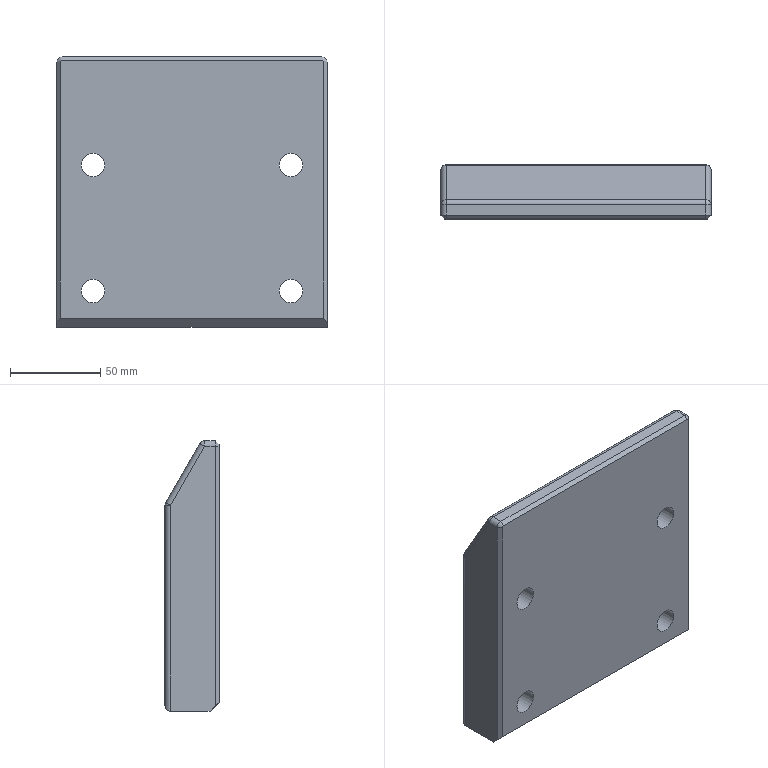Part | NX | features solid 2 | 1 solid | 42 faces | box 150 x 30 x 150 mm | volume 590878 mm3 | cylinder 17 | plane 15 | torus 4 | sphere 4 | cone 2 | commonest cylinder face diameters 6 x9 13 x4 20 x4
STEP:
#1=CARTESIAN_POINT('',(-235.5,-600.,-133.));
#2=VERTEX_POINT('',#1);
#3=CARTESIAN_POINT('',(-235.5,-600.,-275.));
#4=VERTEX_POINT('',#3);
#5=CARTESIAN_POINT('',(-235.5,-600.,-170.));
#6=DIRECTION('',(0.,0.,-1.));
#7=VECTOR('',#6,1000.);
#8=LINE('',#5,#7);
#9=EDGE_CURVE('',#2,#4,#8,.T.);
#10=ORIENTED_EDGE('',*,*,#9,.T.);
#11=CARTESIAN_POINT('',(-233.5,-598.,-277.));
#12=VERTEX_POINT('',#11);
#13=CARTESIAN_POINT('',(-277.167,-641.667,-233.333));
#14=DIRECTION('',(0.5774,0.5774,-0.5774));
#15=VECTOR('',#14,1000.);
#16=LINE('',#13,#15);
#17=EDGE_CURVE('',#12,#4,#16,.F.);
#18=ORIENTED_EDGE('',*,*,#17,.F.);
#19=CARTESIAN_POINT('',(-233.5,-598.,-133.));
#20=VERTEX_POINT('',#19);
#21=CARTESIAN_POINT('',(-233.5,-598.,-43.));
#22=DIRECTION('',(0.,0.,1.));
#23=VECTOR('',#22,1000.);
#24=LINE('',#21,#23);
#25=EDGE_CURVE('',#12,#20,#24,.T.);
#26=ORIENTED_EDGE('',*,*,#25,.T.);
#27=CARTESIAN_POINT('',(-233.5,-598.,-133.));
#28=DIRECTION('',(-0.7071,-0.7071,0.));
#29=VECTOR('',#28,1000.);
#30=LINE('',#27,#29);
#31=EDGE_CURVE('',#20,#2,#30,.T.);
#32=ORIENTED_EDGE('',*,*,#31,.T.);
#33=EDGE_LOOP('',(#10,#18,#26,#32));
#34=FACE_BOUND('',#33,.T.);
#35=CARTESIAN_POINT('',(-235.5,-600.,-40.));
#36=DIRECTION('',(0.7071,-0.7071,0.));
#37=DIRECTION('',(-0.7071,-0.7071,0.));
#38=AXIS2_PLACEMENT_3D('',#35,#36,#37);
#39=PLANE('',#38);
#40=ADVANCED_FACE('',(#34),#39,.T.);
#41=CARTESIAN_POINT('',(-233.5,-573.,-165.804));
#42=VERTEX_POINT('',#41);
#43=CARTESIAN_POINT('',(-233.5,-573.,-280.));
#44=VERTEX_POINT('',#43);
#45=CARTESIAN_POINT('',(-233.5,-573.,-170.));
#46=DIRECTION('',(0.,0.,1.));
#47=VECTOR('',#46,1000.);
#48=LINE('',#45,#47);
#49=EDGE_CURVE('',#42,#44,#48,.F.);
#50=ORIENTED_EDGE('',*,*,#49,.T.);
#51=CARTESIAN_POINT('',(-236.5,-570.,-277.));
#52=VERTEX_POINT('',#51);
#53=CARTESIAN_POINT('',(-236.5,-573.,-277.));
#54=DIRECTION('',(0.7071,0.,0.7071));
#55=DIRECTION('',(-0.7071,0.,0.7071));
#56=AXIS2_PLACEMENT_3D('',#53,#54,#55);
#57=ELLIPSE('',#56,4.243,3.);
#58=EDGE_CURVE('',#44,#52,#57,.T.);
#59=ORIENTED_EDGE('',*,*,#58,.T.);
#60=CARTESIAN_POINT('',(-236.5,-570.,-165.804));
#61=VERTEX_POINT('',#60);
#62=CARTESIAN_POINT('',(-236.5,-570.,-75.));
#63=DIRECTION('',(0.,0.,1.));
#64=VECTOR('',#63,1000.);
#65=LINE('',#62,#64);
#66=EDGE_CURVE('',#52,#61,#65,.T.);
#67=ORIENTED_EDGE('',*,*,#66,.T.);
#68=CARTESIAN_POINT('',(-236.5,-573.,-165.804));
#69=DIRECTION('',(0.,0.,-1.));
#70=DIRECTION('',(-1.,0.,0.));
#71=AXIS2_PLACEMENT_3D('',#68,#69,#70);
#72=CIRCLE('',#71,3.);
#73=EDGE_CURVE('',#42,#61,#72,.F.);
#74=ORIENTED_EDGE('',*,*,#73,.F.);
#75=EDGE_LOOP('',(#50,#59,#67,#74));
#76=FACE_BOUND('',#75,.T.);
#77=CARTESIAN_POINT('',(-236.5,-573.,-170.));
#78=DIRECTION('',(0.,0.,-1.));
#79=DIRECTION('',(1.,0.,0.));
#80=AXIS2_PLACEMENT_3D('',#77,#78,#79);
#81=CYLINDRICAL_SURFACE('',#80,3.);
#82=ADVANCED_FACE('',(#76),#81,.T.);
#83=ORIENTED_EDGE('',*,*,#25,.F.);
#84=CARTESIAN_POINT('',(-233.5,-595.,-280.));
#85=VERTEX_POINT('',#84);
#86=CARTESIAN_POINT('',(-233.5,-600.,-275.));
#87=DIRECTION('',(0.,0.7071,-0.7071));
#88=VECTOR('',#87,1000.);
#89=LINE('',#86,#88);
#90=EDGE_CURVE('',#85,#12,#89,.F.);
#91=ORIENTED_EDGE('',*,*,#90,.F.);
#92=CARTESIAN_POINT('',(-233.5,-600.,-280.));
#93=DIRECTION('',(0.,1.,0.));
#94=VECTOR('',#93,1000.);
#95=LINE('',#92,#94);
#96=EDGE_CURVE('',#85,#44,#95,.T.);
#97=ORIENTED_EDGE('',*,*,#96,.T.);
#98=ORIENTED_EDGE('',*,*,#49,.F.);
#99=CARTESIAN_POINT('',(-233.5,-591.939,-133.));
#100=VERTEX_POINT('',#99);
#101=CARTESIAN_POINT('',(-233.5,-572.598,-166.5));
#102=DIRECTION('',(0.,-0.5,0.866));
#103=VECTOR('',#102,1000.);
#104=LINE('',#101,#103);
#105=EDGE_CURVE('',#100,#42,#104,.F.);
#106=ORIENTED_EDGE('',*,*,#105,.F.);
#107=CARTESIAN_POINT('',(-233.5,-590.207,-133.));
#108=DIRECTION('',(0.,-1.,0.));
#109=VECTOR('',#108,1000.);
#110=LINE('',#107,#109);
#111=EDGE_CURVE('',#20,#100,#110,.F.);
#112=ORIENTED_EDGE('',*,*,#111,.F.);
#113=EDGE_LOOP('',(#83,#91,#97,#98,#106,#112));
#114=FACE_BOUND('',#113,.T.);
#115=CARTESIAN_POINT('',(-233.5,-570.,-40.));
#116=DIRECTION('',(-1.,0.,0.));
#117=DIRECTION('',(0.,0.,-1.));
#118=AXIS2_PLACEMENT_3D('',#115,#116,#117);
#119=PLANE('',#118);
#120=ADVANCED_FACE('',(#114),#119,.F.);
#121=CARTESIAN_POINT('',(-383.5,-598.,-133.));
#122=VERTEX_POINT('',#121);
#123=CARTESIAN_POINT('',(-383.5,-598.,-277.));
#124=VERTEX_POINT('',#123);
#125=CARTESIAN_POINT('',(-383.5,-598.,-40.));
#126=DIRECTION('',(0.,0.,-1.));
#127=VECTOR('',#126,1000.);
#128=LINE('',#125,#127);
#129=EDGE_CURVE('',#122,#124,#128,.T.);
#130=ORIENTED_EDGE('',*,*,#129,.T.);
#131=CARTESIAN_POINT('',(-381.5,-600.,-275.));
#132=VERTEX_POINT('',#131);
#133=CARTESIAN_POINT('',(-341.167,-640.333,-234.667));
#134=DIRECTION('',(-0.5774,0.5774,-0.5774));
#135=VECTOR('',#134,1000.);
#136=LINE('',#133,#135);
#137=EDGE_CURVE('',#132,#124,#136,.T.);
#138=ORIENTED_EDGE('',*,*,#137,.F.);
#139=CARTESIAN_POINT('',(-381.5,-600.,-133.));
#140=VERTEX_POINT('',#139);
#141=CARTESIAN_POINT('',(-381.5,-600.,-40.));
#142=DIRECTION('',(0.,0.,1.));
#143=VECTOR('',#142,1000.);
#144=LINE('',#141,#143);
#145=EDGE_CURVE('',#132,#140,#144,.T.);
#146=ORIENTED_EDGE('',*,*,#145,.T.);
#147=CARTESIAN_POINT('',(-383.5,-598.,-133.));
#148=DIRECTION('',(0.7071,-0.7071,0.));
#149=VECTOR('',#148,1000.);
#150=LINE('',#147,#149);
#151=EDGE_CURVE('',#122,#140,#150,.T.);
#152=ORIENTED_EDGE('',*,*,#151,.F.);
#153=EDGE_LOOP('',(#130,#138,#146,#152));
#154=FACE_BOUND('',#153,.T.);
#155=CARTESIAN_POINT('',(-383.5,-598.,-40.));
#156=DIRECTION('',(0.7071,0.7071,0.));
#157=DIRECTION('',(0.7071,-0.7071,0.));
#158=AXIS2_PLACEMENT_3D('',#155,#156,#157);
#159=PLANE('',#158);
#160=ADVANCED_FACE('',(#154),#159,.F.);
#161=CARTESIAN_POINT('',(-380.5,-570.,-165.804));
#162=VERTEX_POINT('',#161);
#163=CARTESIAN_POINT('',(-380.5,-570.,-277.));
#164=VERTEX_POINT('',#163);
#165=CARTESIAN_POINT('',(-380.5,-570.,-170.));
#166=DIRECTION('',(0.,0.,1.));
#167=VECTOR('',#166,1000.);
#168=LINE('',#165,#167);
#169=EDGE_CURVE('',#162,#164,#168,.F.);
#170=ORIENTED_EDGE('',*,*,#169,.T.);
#171=CARTESIAN_POINT('',(-383.5,-573.,-280.));
#172=VERTEX_POINT('',#171);
#173=CARTESIAN_POINT('',(-380.5,-573.,-277.));
#174=DIRECTION('',(0.7071,0.,-0.7071));
#175=DIRECTION('',(-0.7071,0.,-0.7071));
#176=AXIS2_PLACEMENT_3D('',#173,#174,#175);
#177=ELLIPSE('',#176,4.243,3.);
#178=EDGE_CURVE('',#172,#164,#177,.T.);
#179=ORIENTED_EDGE('',*,*,#178,.F.);
#180=CARTESIAN_POINT('',(-383.5,-573.,-165.804));
#181=VERTEX_POINT('',#180);
#182=CARTESIAN_POINT('',(-383.5,-573.,-40.));
#183=DIRECTION('',(0.,0.,1.));
#184=VECTOR('',#183,1000.);
#185=LINE('',#182,#184);
#186=EDGE_CURVE('',#172,#181,#185,.T.);
#187=ORIENTED_EDGE('',*,*,#186,.T.);
#188=CARTESIAN_POINT('',(-380.5,-573.,-165.804));
#189=DIRECTION('',(0.,0.,-1.));
#190=DIRECTION('',(-1.,0.,0.));
#191=AXIS2_PLACEMENT_3D('',#188,#189,#190);
#192=CIRCLE('',#191,3.);
#193=EDGE_CURVE('',#162,#181,#192,.F.);
#194=ORIENTED_EDGE('',*,*,#193,.F.);
#195=EDGE_LOOP('',(#170,#179,#187,#194));
#196=FACE_BOUND('',#195,.T.);
#197=CARTESIAN_POINT('',(-380.5,-573.,-40.));
#198=DIRECTION('',(0.,0.,1.));
#199=DIRECTION('',(-1.,0.,0.));
#200=AXIS2_PLACEMENT_3D('',#197,#198,#199);
#201=CYLINDRICAL_SURFACE('',#200,3.);
#202=ADVANCED_FACE('',(#196),#201,.T.);
#203=ORIENTED_EDGE('',*,*,#186,.F.);
#204=CARTESIAN_POINT('',(-383.5,-595.,-280.));
#205=VERTEX_POINT('',#204);
#206=CARTESIAN_POINT('',(-383.5,-600.,-280.));
#207=DIRECTION('',(0.,1.,0.));
#208=VECTOR('',#207,1000.);
#209=LINE('',#206,#208);
#210=EDGE_CURVE('',#205,#172,#209,.T.);
#211=ORIENTED_EDGE('',*,*,#210,.F.);
#212=CARTESIAN_POINT('',(-383.5,-647.5,-227.5));
#213=DIRECTION('',(0.,-0.7071,0.7071));
#214=VECTOR('',#213,1000.);
#215=LINE('',#212,#214);
#216=EDGE_CURVE('',#124,#205,#215,.F.);
#217=ORIENTED_EDGE('',*,*,#216,.F.);
#218=ORIENTED_EDGE('',*,*,#129,.F.);
#219=CARTESIAN_POINT('',(-383.5,-591.939,-133.));
#220=VERTEX_POINT('',#219);
#221=CARTESIAN_POINT('',(-383.5,-570.,-133.));
#222=DIRECTION('',(0.,-1.,0.));
#223=VECTOR('',#222,1000.);
#224=LINE('',#221,#223);
#225=EDGE_CURVE('',#220,#122,#224,.T.);
#226=ORIENTED_EDGE('',*,*,#225,.F.);
#227=CARTESIAN_POINT('',(-383.5,-587.754,-140.25));
#228=DIRECTION('',(0.,-0.5,0.866));
#229=VECTOR('',#228,1000.);
#230=LINE('',#227,#229);
#231=EDGE_CURVE('',#181,#220,#230,.T.);
#232=ORIENTED_EDGE('',*,*,#231,.F.);
#233=EDGE_LOOP('',(#203,#211,#217,#218,#226,#232));
#234=FACE_BOUND('',#233,.T.);
#235=CARTESIAN_POINT('',(-383.5,-570.,-40.));
#236=DIRECTION('',(-1.,0.,0.));
#237=DIRECTION('',(0.,0.,-1.));
#238=AXIS2_PLACEMENT_3D('',#235,#236,#237);
#239=PLANE('',#238);
#240=ADVANCED_FACE('',(#234),#239,.T.);
#241=CARTESIAN_POINT('',(-260.,-600.,-260.));
#242=VERTEX_POINT('',#241);
#243=CARTESIAN_POINT('',(-253.5,-600.,-260.));
#244=DIRECTION('',(0.,1.,0.));
#245=DIRECTION('',(-1.,0.,0.));
#246=AXIS2_PLACEMENT_3D('',#243,#244,#245);
#247=CIRCLE('',#246,6.5);
#248=EDGE_CURVE('',#242,#242,#247,.T.);
#249=ORIENTED_EDGE('',*,*,#248,.T.);
#250=EDGE_LOOP('',(#249));
#251=FACE_BOUND('',#250,.T.);
#252=CARTESIAN_POINT('',(-370.,-600.,-260.));
#253=VERTEX_POINT('',#252);
#254=CARTESIAN_POINT('',(-363.5,-600.,-260.));
#255=DIRECTION('',(0.,1.,0.));
#256=DIRECTION('',(-1.,0.,0.));
#257=AXIS2_PLACEMENT_3D('',#254,#255,#256);
#258=CIRCLE('',#257,6.5);
#259=EDGE_CURVE('',#253,#253,#258,.T.);
#260=ORIENTED_EDGE('',*,*,#259,.T.);
#261=EDGE_LOOP('',(#260));
#262=FACE_BOUND('',#261,.T.);
#263=ORIENTED_EDGE('',*,*,#145,.F.);
#264=CARTESIAN_POINT('',(-271.,-600.,-275.));
#265=DIRECTION('',(-1.,0.,0.));
#266=VECTOR('',#265,1000.);
#267=LINE('',#264,#266);
#268=EDGE_CURVE('',#4,#132,#267,.T.);
#269=ORIENTED_EDGE('',*,*,#268,.F.);
#270=ORIENTED_EDGE('',*,*,#9,.F.);
#271=CARTESIAN_POINT('',(-236.5,-600.,-132.));
#272=VERTEX_POINT('',#271);
#273=CARTESIAN_POINT('',(-236.5,-600.,-133.));
#274=DIRECTION('',(0.,1.,0.));
#275=DIRECTION('',(0.,0.,1.));
#276=AXIS2_PLACEMENT_3D('',#273,#274,#275);
#277=CIRCLE('',#276,1.);
#278=EDGE_CURVE('',#272,#2,#277,.T.);
#279=ORIENTED_EDGE('',*,*,#278,.F.);
#280=CARTESIAN_POINT('',(-380.5,-600.,-132.));
#281=VERTEX_POINT('',#280);
#282=CARTESIAN_POINT('',(-271.,-600.,-132.));
#283=DIRECTION('',(1.,0.,0.));
#284=VECTOR('',#283,1000.);
#285=LINE('',#282,#284);
#286=EDGE_CURVE('',#281,#272,#285,.T.);
#287=ORIENTED_EDGE('',*,*,#286,.F.);
#288=CARTESIAN_POINT('',(-380.5,-600.,-133.));
#289=DIRECTION('',(0.,1.,0.));
#290=DIRECTION('',(0.,0.,1.));
#291=AXIS2_PLACEMENT_3D('',#288,#289,#290);
#292=CIRCLE('',#291,1.);
#293=EDGE_CURVE('',#140,#281,#292,.T.);
#294=ORIENTED_EDGE('',*,*,#293,.F.);
#295=EDGE_LOOP('',(#263,#269,#270,#279,#287,#294));
#296=FACE_BOUND('',#295,.T.);
#297=CARTESIAN_POINT('',(-260.,-600.,-190.));
#298=VERTEX_POINT('',#297);
#299=CARTESIAN_POINT('',(-253.5,-600.,-190.));
#300=DIRECTION('',(0.,1.,0.));
#301=DIRECTION('',(-1.,0.,0.));
#302=AXIS2_PLACEMENT_3D('',#299,#300,#301);
#303=CIRCLE('',#302,6.5);
#304=EDGE_CURVE('',#298,#298,#303,.T.);
#305=ORIENTED_EDGE('',*,*,#304,.T.);
#306=EDGE_LOOP('',(#305));
#307=FACE_BOUND('',#306,.T.);
#308=CARTESIAN_POINT('',(-370.,-600.,-190.));
#309=VERTEX_POINT('',#308);
#310=CARTESIAN_POINT('',(-363.5,-600.,-190.));
#311=DIRECTION('',(0.,1.,0.));
#312=DIRECTION('',(-1.,0.,0.));
#313=AXIS2_PLACEMENT_3D('',#310,#311,#312);
#314=CIRCLE('',#313,6.5);
#315=EDGE_CURVE('',#309,#309,#314,.T.);
#316=ORIENTED_EDGE('',*,*,#315,.T.);
#317=EDGE_LOOP('',(#316));
#318=FACE_BOUND('',#317,.T.);
#319=CARTESIAN_POINT('',(-271.,-600.,-40.));
#320=DIRECTION('',(0.,-1.,0.));
#321=DIRECTION('',(0.,0.,1.));
#322=AXIS2_PLACEMENT_3D('',#319,#320,#321);
#323=PLANE('',#322);
#324=ADVANCED_FACE('',(#251,#262,#296,#307,#318),#323,.T.);
#325=CARTESIAN_POINT('',(-240.5,-570.,-260.));
#326=VERTEX_POINT('',#325);
#327=CARTESIAN_POINT('',(-253.5,-570.,-260.));
#328=DIRECTION('',(0.,-1.,0.));
#329=DIRECTION('',(1.,0.,0.));
#330=AXIS2_PLACEMENT_3D('',#327,#328,#329);
#331=CIRCLE('',#330,13.);
#332=EDGE_CURVE('',#326,#326,#331,.F.);
#333=ORIENTED_EDGE('',*,*,#332,.F.);
#334=EDGE_LOOP('',(#333));
#335=FACE_BOUND('',#334,.T.);
#336=CARTESIAN_POINT('',(-350.5,-570.,-260.));
#337=VERTEX_POINT('',#336);
#338=CARTESIAN_POINT('',(-363.5,-570.,-260.));
#339=DIRECTION('',(0.,-1.,0.));
#340=DIRECTION('',(1.,0.,0.));
#341=AXIS2_PLACEMENT_3D('',#338,#339,#340);
#342=CIRCLE('',#341,13.);
#343=EDGE_CURVE('',#337,#337,#342,.F.);
#344=ORIENTED_EDGE('',*,*,#343,.F.);
#345=EDGE_LOOP('',(#344));
#346=FACE_BOUND('',#345,.T.);
#347=ORIENTED_EDGE('',*,*,#66,.F.);
#348=CARTESIAN_POINT('',(-271.,-570.,-277.));
#349=DIRECTION('',(-1.,0.,0.));
#350=VECTOR('',#349,1000.);
#351=LINE('',#348,#350);
#352=EDGE_CURVE('',#164,#52,#351,.F.);
#353=ORIENTED_EDGE('',*,*,#352,.F.);
#354=ORIENTED_EDGE('',*,*,#169,.F.);
#355=CARTESIAN_POINT('',(-271.,-570.,-165.804));
#356=DIRECTION('',(-1.,0.,0.));
#357=VECTOR('',#356,1000.);
#358=LINE('',#355,#357);
#359=EDGE_CURVE('',#61,#162,#358,.T.);
#360=ORIENTED_EDGE('',*,*,#359,.F.);
#361=EDGE_LOOP('',(#347,#353,#354,#360));
#362=FACE_BOUND('',#361,.T.);
#363=CARTESIAN_POINT('',(-240.5,-570.,-190.));
#364=VERTEX_POINT('',#363);
#365=CARTESIAN_POINT('',(-253.5,-570.,-190.));
#366=DIRECTION('',(0.,-1.,0.));
#367=DIRECTION('',(1.,0.,0.));
#368=AXIS2_PLACEMENT_3D('',#365,#366,#367);
#369=CIRCLE('',#368,13.);
#370=EDGE_CURVE('',#364,#364,#369,.F.);
#371=ORIENTED_EDGE('',*,*,#370,.F.);
#372=EDGE_LOOP('',(#371));
#373=FACE_BOUND('',#372,.T.);
#374=CARTESIAN_POINT('',(-350.5,-570.,-190.));
#375=VERTEX_POINT('',#374);
#376=CARTESIAN_POINT('',(-363.5,-570.,-190.));
#377=DIRECTION('',(0.,-1.,0.));
#378=DIRECTION('',(1.,0.,0.));
#379=AXIS2_PLACEMENT_3D('',#376,#377,#378);
#380=CIRCLE('',#379,13.);
#381=EDGE_CURVE('',#375,#375,#380,.F.);
#382=ORIENTED_EDGE('',*,*,#381,.F.);
#383=EDGE_LOOP('',(#382));
#384=FACE_BOUND('',#383,.T.);
#385=CARTESIAN_POINT('',(-271.,-570.,-170.));
#386=DIRECTION('',(0.,1.,0.));
#387=DIRECTION('',(1.,0.,0.));
#388=AXIS2_PLACEMENT_3D('',#385,#386,#387);
#389=PLANE('',#388);
#390=ADVANCED_FACE('',(#335,#346,#362,#373,#384),#389,.T.);
#391=CARTESIAN_POINT('',(-243.5,-573.,-260.));
#392=VERTEX_POINT('',#391);
#393=CARTESIAN_POINT('',(-253.5,-573.,-260.));
#394=DIRECTION('',(0.,-1.,0.));
#395=DIRECTION('',(1.,0.,0.));
#396=AXIS2_PLACEMENT_3D('',#393,#394,#395);
#397=CIRCLE('',#396,10.);
#398=EDGE_CURVE('',#392,#392,#397,.T.);
#399=ORIENTED_EDGE('',*,*,#398,.F.);
#400=EDGE_LOOP('',(#399));
#401=FACE_BOUND('',#400,.T.);
#402=CARTESIAN_POINT('',(-263.5,-585.,-260.));
#403=VERTEX_POINT('',#402);
#404=CARTESIAN_POINT('',(-253.5,-585.,-260.));
#405=DIRECTION('',(0.,1.,0.));
#406=DIRECTION('',(-1.,0.,0.));
#407=AXIS2_PLACEMENT_3D('',#404,#405,#406);
#408=CIRCLE('',#407,10.);
#409=EDGE_CURVE('',#403,#403,#408,.T.);
#410=ORIENTED_EDGE('',*,*,#409,.F.);
#411=EDGE_LOOP('',(#410));
#412=FACE_BOUND('',#411,.T.);
#413=CARTESIAN_POINT('',(-253.5,-570.,-260.));
#414=DIRECTION('',(0.,-1.,0.));
#415=DIRECTION('',(-1.,0.,0.));
#416=AXIS2_PLACEMENT_3D('',#413,#414,#415);
#417=CYLINDRICAL_SURFACE('',#416,10.);
#418=ADVANCED_FACE('',(#401,#412),#417,.F.);
#419=CARTESIAN_POINT('',(-353.5,-573.,-260.));
#420=VERTEX_POINT('',#419);
#421=CARTESIAN_POINT('',(-363.5,-573.,-260.));
#422=DIRECTION('',(0.,-1.,0.));
#423=DIRECTION('',(1.,0.,0.));
#424=AXIS2_PLACEMENT_3D('',#421,#422,#423);
#425=CIRCLE('',#424,10.);
#426=EDGE_CURVE('',#420,#420,#425,.T.);
#427=ORIENTED_EDGE('',*,*,#426,.F.);
#428=EDGE_LOOP('',(#427));
#429=FACE_BOUND('',#428,.T.);
#430=CARTESIAN_POINT('',(-373.5,-585.,-260.));
#431=VERTEX_POINT('',#430);
#432=CARTESIAN_POINT('',(-363.5,-585.,-260.));
#433=DIRECTION('',(0.,1.,0.));
#434=DIRECTION('',(-1.,0.,0.));
#435=AXIS2_PLACEMENT_3D('',#432,#433,#434);
#436=CIRCLE('',#435,10.);
#437=EDGE_CURVE('',#431,#431,#436,.T.);
#438=ORIENTED_EDGE('',*,*,#437,.F.);
#439=EDGE_LOOP('',(#438));
#440=FACE_BOUND('',#439,.T.);
#441=CARTESIAN_POINT('',(-363.5,-570.,-260.));
#442=DIRECTION('',(0.,-1.,0.));
#443=DIRECTION('',(-1.,0.,0.));
#444=AXIS2_PLACEMENT_3D('',#441,#442,#443);
#445=CYLINDRICAL_SURFACE('',#444,10.);
#446=ADVANCED_FACE('',(#429,#440),#445,.F.);
#447=CARTESIAN_POINT('',(-260.,-585.,-260.));
#448=VERTEX_POINT('',#447);
#449=CARTESIAN_POINT('',(-253.5,-585.,-260.));
#450=DIRECTION('',(0.,1.,0.));
#451=DIRECTION('',(-1.,0.,0.));
#452=AXIS2_PLACEMENT_3D('',#449,#450,#451);
#453=CIRCLE('',#452,6.5);
#454=EDGE_CURVE('',#448,#448,#453,.T.);
#455=ORIENTED_EDGE('',*,*,#454,.F.);
#456=EDGE_LOOP('',(#455));
#457=FACE_BOUND('',#456,.T.);
#458=ORIENTED_EDGE('',*,*,#409,.T.);
#459=EDGE_LOOP('',(#458));
#460=FACE_BOUND('',#459,.T.);
#461=CARTESIAN_POINT('',(-288.5,-585.,-150.));
#462=DIRECTION('',(0.,-1.,0.));
#463=DIRECTION('',(-1.,0.,0.));
#464=AXIS2_PLACEMENT_3D('',#461,#462,#463);
#465=PLANE('',#464);
#466=ADVANCED_FACE('',(#457,#460),#465,.F.);
#467=CARTESIAN_POINT('',(-370.,-585.,-260.));
#468=VERTEX_POINT('',#467);
#469=CARTESIAN_POINT('',(-363.5,-585.,-260.));
#470=DIRECTION('',(0.,1.,0.));
#471=DIRECTION('',(-1.,0.,0.));
#472=AXIS2_PLACEMENT_3D('',#469,#470,#471);
#473=CIRCLE('',#472,6.5);
#474=EDGE_CURVE('',#468,#468,#473,.T.);
#475=ORIENTED_EDGE('',*,*,#474,.F.);
#476=EDGE_LOOP('',(#475));
#477=FACE_BOUND('',#476,.T.);
#478=ORIENTED_EDGE('',*,*,#437,.T.);
#479=EDGE_LOOP('',(#478));
#480=FACE_BOUND('',#479,.T.);
#481=CARTESIAN_POINT('',(-328.5,-585.,-150.));
#482=DIRECTION('',(0.,-1.,0.));
#483=DIRECTION('',(-1.,0.,0.));
#484=AXIS2_PLACEMENT_3D('',#481,#482,#483);
#485=PLANE('',#484);
#486=ADVANCED_FACE('',(#477,#480),#485,.F.);
#487=ORIENTED_EDGE('',*,*,#398,.T.);
#488=EDGE_LOOP('',(#487));
#489=FACE_BOUND('',#488,.T.);
#490=ORIENTED_EDGE('',*,*,#332,.T.);
#491=EDGE_LOOP('',(#490));
#492=FACE_BOUND('',#491,.T.);
#493=CARTESIAN_POINT('',(-253.5,-573.,-260.));
#494=DIRECTION('',(0.,1.,0.));
#495=DIRECTION('',(1.,0.,0.));
#496=AXIS2_PLACEMENT_3D('',#493,#494,#495);
#497=TOROIDAL_SURFACE('',#496,13.,3.);
#498=ADVANCED_FACE('',(#489,#492),#497,.T.);
#499=ORIENTED_EDGE('',*,*,#426,.T.);
#500=EDGE_LOOP('',(#499));
#501=FACE_BOUND('',#500,.T.);
#502=ORIENTED_EDGE('',*,*,#343,.T.);
#503=EDGE_LOOP('',(#502));
#504=FACE_BOUND('',#503,.T.);
#505=CARTESIAN_POINT('',(-363.5,-573.,-260.));
#506=DIRECTION('',(0.,1.,0.));
#507=DIRECTION('',(1.,0.,0.));
#508=AXIS2_PLACEMENT_3D('',#505,#506,#507);
#509=TOROIDAL_SURFACE('',#508,13.,3.);
#510=ADVANCED_FACE('',(#501,#504),#509,.T.);
#511=ORIENTED_EDGE('',*,*,#248,.F.);
#512=EDGE_LOOP('',(#511));
#513=FACE_BOUND('',#512,.T.);
#514=ORIENTED_EDGE('',*,*,#454,.T.);
#515=EDGE_LOOP('',(#514));
#516=FACE_BOUND('',#515,.T.);
#517=CARTESIAN_POINT('',(-253.5,-600.,-260.));
#518=DIRECTION('',(0.,-1.,0.));
#519=DIRECTION('',(-1.,0.,0.));
#520=AXIS2_PLACEMENT_3D('',#517,#518,#519);
#521=CYLINDRICAL_SURFACE('',#520,6.5);
#522=ADVANCED_FACE('',(#513,#516),#521,.F.);
#523=ORIENTED_EDGE('',*,*,#259,.F.);
#524=EDGE_LOOP('',(#523));
#525=FACE_BOUND('',#524,.T.);
#526=ORIENTED_EDGE('',*,*,#474,.T.);
#527=EDGE_LOOP('',(#526));
#528=FACE_BOUND('',#527,.T.);
#529=CARTESIAN_POINT('',(-363.5,-600.,-260.));
#530=DIRECTION('',(0.,-1.,0.));
#531=DIRECTION('',(-1.,0.,0.));
#532=AXIS2_PLACEMENT_3D('',#529,#530,#531);
#533=CYLINDRICAL_SURFACE('',#532,6.5);
#534=ADVANCED_FACE('',(#525,#528),#533,.F.);
#535=ORIENTED_EDGE('',*,*,#210,.T.);
#536=CARTESIAN_POINT('',(-271.,-573.,-280.));
#537=DIRECTION('',(-1.,0.,0.));
#538=VECTOR('',#537,1000.);
#539=LINE('',#536,#538);
#540=EDGE_CURVE('',#44,#172,#539,.T.);
#541=ORIENTED_EDGE('',*,*,#540,.F.);
#542=ORIENTED_EDGE('',*,*,#96,.F.);
#543=CARTESIAN_POINT('',(-271.,-595.,-280.));
#544=DIRECTION('',(1.,0.,0.));
#545=VECTOR('',#544,1000.);
#546=LINE('',#543,#545);
#547=EDGE_CURVE('',#205,#85,#546,.T.);
#548=ORIENTED_EDGE('',*,*,#547,.F.);
#549=EDGE_LOOP('',(#535,#541,#542,#548));
#550=FACE_BOUND('',#549,.T.);
#551=CARTESIAN_POINT('',(-271.,-600.,-280.));
#552=DIRECTION('',(0.,0.,-1.));
#553=DIRECTION('',(1.,0.,0.));
#554=AXIS2_PLACEMENT_3D('',#551,#552,#553);
#555=PLANE('',#554);
#556=ADVANCED_FACE('',(#550),#555,.T.);
#557=ORIENTED_EDGE('',*,*,#58,.F.);
#558=ORIENTED_EDGE('',*,*,#540,.T.);
#559=ORIENTED_EDGE('',*,*,#178,.T.);
#560=ORIENTED_EDGE('',*,*,#352,.T.);
#561=EDGE_LOOP('',(#557,#558,#559,#560));
#562=FACE_BOUND('',#561,.T.);
#563=CARTESIAN_POINT('',(-271.,-573.,-277.));
#564=DIRECTION('',(-1.,0.,0.));
#565=DIRECTION('',(0.,0.,-1.));
#566=AXIS2_PLACEMENT_3D('',#563,#564,#565);
#567=CYLINDRICAL_SURFACE('',#566,3.);
#568=ADVANCED_FACE('',(#562),#567,.T.);
#569=ORIENTED_EDGE('',*,*,#90,.T.);
#570=ORIENTED_EDGE('',*,*,#17,.T.);
#571=ORIENTED_EDGE('',*,*,#268,.T.);
#572=ORIENTED_EDGE('',*,*,#137,.T.);
#573=ORIENTED_EDGE('',*,*,#216,.T.);
#574=ORIENTED_EDGE('',*,*,#547,.T.);
#575=EDGE_LOOP('',(#569,#570,#571,#572,#573,#574));
#576=FACE_BOUND('',#575,.T.);
#577=CARTESIAN_POINT('',(-271.,-600.,-275.));
#578=DIRECTION('',(0.,0.7071,0.7071));
#579=DIRECTION('',(0.,0.7071,-0.7071));
#580=AXIS2_PLACEMENT_3D('',#577,#578,#579);
#581=PLANE('',#580);
#582=ADVANCED_FACE('',(#576),#581,.F.);
#583=CARTESIAN_POINT('',(-236.5,-570.402,-164.304));
#584=VERTEX_POINT('',#583);
#585=CARTESIAN_POINT('',(-236.5,-589.341,-131.5));
#586=VERTEX_POINT('',#585);
#587=CARTESIAN_POINT('',(-236.5,-590.207,-130.));
#588=DIRECTION('',(0.,-0.5,0.866));
#589=VECTOR('',#588,1000.);
#590=LINE('',#587,#589);
#591=EDGE_CURVE('',#584,#586,#590,.T.);
#592=ORIENTED_EDGE('',*,*,#591,.F.);
#593=CARTESIAN_POINT('',(-380.5,-570.402,-164.304));
#594=VERTEX_POINT('',#593);
#595=CARTESIAN_POINT('',(-271.,-570.402,-164.304));
#596=DIRECTION('',(-1.,0.,0.));
#597=VECTOR('',#596,1000.);
#598=LINE('',#595,#597);
#599=EDGE_CURVE('',#594,#584,#598,.F.);
#600=ORIENTED_EDGE('',*,*,#599,.F.);
#601=CARTESIAN_POINT('',(-380.5,-589.341,-131.5));
#602=VERTEX_POINT('',#601);
#603=CARTESIAN_POINT('',(-380.5,-570.,-165.));
#604=DIRECTION('',(0.,-0.5,0.866));
#605=VECTOR('',#604,1000.);
#606=LINE('',#603,#605);
#607=EDGE_CURVE('',#602,#594,#606,.F.);
#608=ORIENTED_EDGE('',*,*,#607,.F.);
#609=CARTESIAN_POINT('',(-271.,-589.341,-131.5));
#610=DIRECTION('',(-1.,0.,0.));
#611=VECTOR('',#610,1000.);
#612=LINE('',#609,#611);
#613=EDGE_CURVE('',#586,#602,#612,.T.);
#614=ORIENTED_EDGE('',*,*,#613,.F.);
#615=EDGE_LOOP('',(#592,#600,#608,#614));
#616=FACE_BOUND('',#615,.T.);
#617=CARTESIAN_POINT('',(-271.,-570.,-165.));
#618=DIRECTION('',(0.,0.866,0.5));
#619=DIRECTION('',(0.,0.5,-0.866));
#620=AXIS2_PLACEMENT_3D('',#617,#618,#619);
#621=PLANE('',#620);
#622=ADVANCED_FACE('',(#616),#621,.T.);
#623=CARTESIAN_POINT('',(-236.5,-591.939,-130.));
#624=VERTEX_POINT('',#623);
#625=CARTESIAN_POINT('',(-236.5,-598.,-130.));
#626=VERTEX_POINT('',#625);
#627=CARTESIAN_POINT('',(-236.5,-600.,-130.));
#628=DIRECTION('',(0.,-1.,0.));
#629=VECTOR('',#628,1000.);
#630=LINE('',#627,#629);
#631=EDGE_CURVE('',#624,#626,#630,.T.);
#632=ORIENTED_EDGE('',*,*,#631,.F.);
#633=CARTESIAN_POINT('',(-380.5,-591.939,-130.));
#634=VERTEX_POINT('',#633);
#635=CARTESIAN_POINT('',(-271.,-591.939,-130.));
#636=DIRECTION('',(-1.,0.,0.));
#637=VECTOR('',#636,1000.);
#638=LINE('',#635,#637);
#639=EDGE_CURVE('',#634,#624,#638,.F.);
#640=ORIENTED_EDGE('',*,*,#639,.F.);
#641=CARTESIAN_POINT('',(-380.5,-598.,-130.));
#642=VERTEX_POINT('',#641);
#643=CARTESIAN_POINT('',(-380.5,-590.207,-130.));
#644=DIRECTION('',(0.,-1.,0.));
#645=VECTOR('',#644,1000.);
#646=LINE('',#643,#645);
#647=EDGE_CURVE('',#642,#634,#646,.F.);
#648=ORIENTED_EDGE('',*,*,#647,.F.);
#649=CARTESIAN_POINT('',(-271.,-598.,-130.));
#650=DIRECTION('',(-1.,0.,0.));
#651=VECTOR('',#650,1000.);
#652=LINE('',#649,#651);
#653=EDGE_CURVE('',#626,#642,#652,.T.);
#654=ORIENTED_EDGE('',*,*,#653,.F.);
#655=EDGE_LOOP('',(#632,#640,#648,#654));
#656=FACE_BOUND('',#655,.T.);
#657=CARTESIAN_POINT('',(-271.,-590.207,-130.));
#658=DIRECTION('',(0.,0.,1.));
#659=DIRECTION('',(-1.,0.,0.));
#660=AXIS2_PLACEMENT_3D('',#657,#658,#659);
#661=PLANE('',#660);
#662=ADVANCED_FACE('',(#656),#661,.T.);
#663=ORIENTED_EDGE('',*,*,#315,.F.);
#664=EDGE_LOOP('',(#663));
#665=FACE_BOUND('',#664,.T.);
#666=CARTESIAN_POINT('',(-370.,-585.,-190.));
#667=VERTEX_POINT('',#666);
#668=CARTESIAN_POINT('',(-363.5,-585.,-190.));
#669=DIRECTION('',(0.,1.,0.));
#670=DIRECTION('',(-1.,0.,0.));
#671=AXIS2_PLACEMENT_3D('',#668,#669,#670);
#672=CIRCLE('',#671,6.5);
#673=EDGE_CURVE('',#667,#667,#672,.T.);
#674=ORIENTED_EDGE('',*,*,#673,.T.);
#675=EDGE_LOOP('',(#674));
#676=FACE_BOUND('',#675,.T.);
#677=CARTESIAN_POINT('',(-363.5,-600.,-190.));
#678=DIRECTION('',(0.,-1.,0.));
#679=DIRECTION('',(-1.,0.,0.));
#680=AXIS2_PLACEMENT_3D('',#677,#678,#679);
#681=CYLINDRICAL_SURFACE('',#680,6.5);
#682=ADVANCED_FACE('',(#665,#676),#681,.F.);
#683=ORIENTED_EDGE('',*,*,#673,.F.);
#684=EDGE_LOOP('',(#683));
#685=FACE_BOUND('',#684,.T.);
#686=CARTESIAN_POINT('',(-373.5,-585.,-190.));
#687=VERTEX_POINT('',#686);
#688=CARTESIAN_POINT('',(-363.5,-585.,-190.));
#689=DIRECTION('',(0.,1.,0.));
#690=DIRECTION('',(-1.,0.,0.));
#691=AXIS2_PLACEMENT_3D('',#688,#689,#690);
#692=CIRCLE('',#691,10.);
#693=EDGE_CURVE('',#687,#687,#692,.T.);
#694=ORIENTED_EDGE('',*,*,#693,.T.);
#695=EDGE_LOOP('',(#694));
#696=FACE_BOUND('',#695,.T.);
#697=CARTESIAN_POINT('',(-328.5,-585.,-190.));
#698=DIRECTION('',(0.,-1.,0.));
#699=DIRECTION('',(-1.,0.,0.));
#700=AXIS2_PLACEMENT_3D('',#697,#698,#699);
#701=PLANE('',#700);
#702=ADVANCED_FACE('',(#685,#696),#701,.F.);
#703=CARTESIAN_POINT('',(-353.5,-573.,-190.));
#704=VERTEX_POINT('',#703);
#705=CARTESIAN_POINT('',(-363.5,-573.,-190.));
#706=DIRECTION('',(0.,-1.,0.));
#707=DIRECTION('',(1.,0.,0.));
#708=AXIS2_PLACEMENT_3D('',#705,#706,#707);
#709=CIRCLE('',#708,10.);
#710=EDGE_CURVE('',#704,#704,#709,.T.);
#711=ORIENTED_EDGE('',*,*,#710,.F.);
#712=EDGE_LOOP('',(#711));
#713=FACE_BOUND('',#712,.T.);
#714=ORIENTED_EDGE('',*,*,#693,.F.);
#715=EDGE_LOOP('',(#714));
#716=FACE_BOUND('',#715,.T.);
#717=CARTESIAN_POINT('',(-363.5,-570.,-190.));
#718=DIRECTION('',(0.,-1.,0.));
#719=DIRECTION('',(-1.,0.,0.));
#720=AXIS2_PLACEMENT_3D('',#717,#718,#719);
#721=CYLINDRICAL_SURFACE('',#720,10.);
#722=ADVANCED_FACE('',(#713,#716),#721,.F.);
#723=ORIENTED_EDGE('',*,*,#304,.F.);
#724=EDGE_LOOP('',(#723));
#725=FACE_BOUND('',#724,.T.);
#726=CARTESIAN_POINT('',(-260.,-585.,-190.));
#727=VERTEX_POINT('',#726);
#728=CARTESIAN_POINT('',(-253.5,-585.,-190.));
#729=DIRECTION('',(0.,1.,0.));
#730=DIRECTION('',(-1.,0.,0.));
#731=AXIS2_PLACEMENT_3D('',#728,#729,#730);
#732=CIRCLE('',#731,6.5);
#733=EDGE_CURVE('',#727,#727,#732,.T.);
#734=ORIENTED_EDGE('',*,*,#733,.T.);
#735=EDGE_LOOP('',(#734));
#736=FACE_BOUND('',#735,.T.);
#737=CARTESIAN_POINT('',(-253.5,-600.,-190.));
#738=DIRECTION('',(0.,-1.,0.));
#739=DIRECTION('',(-1.,0.,0.));
#740=AXIS2_PLACEMENT_3D('',#737,#738,#739);
#741=CYLINDRICAL_SURFACE('',#740,6.5);
#742=ADVANCED_FACE('',(#725,#736),#741,.F.);
#743=ORIENTED_EDGE('',*,*,#733,.F.);
#744=EDGE_LOOP('',(#743));
#745=FACE_BOUND('',#744,.T.);
#746=CARTESIAN_POINT('',(-263.5,-585.,-190.));
#747=VERTEX_POINT('',#746);
#748=CARTESIAN_POINT('',(-253.5,-585.,-190.));
#749=DIRECTION('',(0.,1.,0.));
#750=DIRECTION('',(-1.,0.,0.));
#751=AXIS2_PLACEMENT_3D('',#748,#749,#750);
#752=CIRCLE('',#751,10.);
#753=EDGE_CURVE('',#747,#747,#752,.T.);
#754=ORIENTED_EDGE('',*,*,#753,.T.);
#755=EDGE_LOOP('',(#754));
#756=FACE_BOUND('',#755,.T.);
#757=CARTESIAN_POINT('',(-288.5,-585.,-190.));
#758=DIRECTION('',(0.,-1.,0.));
#759=DIRECTION('',(-1.,0.,0.));
#760=AXIS2_PLACEMENT_3D('',#757,#758,#759);
#761=PLANE('',#760);
#762=ADVANCED_FACE('',(#745,#756),#761,.F.);
#763=CARTESIAN_POINT('',(-243.5,-573.,-190.));
#764=VERTEX_POINT('',#763);
#765=CARTESIAN_POINT('',(-253.5,-573.,-190.));
#766=DIRECTION('',(0.,-1.,0.));
#767=DIRECTION('',(1.,0.,0.));
#768=AXIS2_PLACEMENT_3D('',#765,#766,#767);
#769=CIRCLE('',#768,10.);
#770=EDGE_CURVE('',#764,#764,#769,.T.);
#771=ORIENTED_EDGE('',*,*,#770,.F.);
#772=EDGE_LOOP('',(#771));
#773=FACE_BOUND('',#772,.T.);
#774=ORIENTED_EDGE('',*,*,#753,.F.);
#775=EDGE_LOOP('',(#774));
#776=FACE_BOUND('',#775,.T.);
#777=CARTESIAN_POINT('',(-253.5,-570.,-190.));
#778=DIRECTION('',(0.,-1.,0.));
#779=DIRECTION('',(-1.,0.,0.));
#780=AXIS2_PLACEMENT_3D('',#777,#778,#779);
#781=CYLINDRICAL_SURFACE('',#780,10.);
#782=ADVANCED_FACE('',(#773,#776),#781,.F.);
#783=ORIENTED_EDGE('',*,*,#770,.T.);
#784=EDGE_LOOP('',(#783));
#785=FACE_BOUND('',#784,.T.);
#786=ORIENTED_EDGE('',*,*,#370,.T.);
#787=EDGE_LOOP('',(#786));
#788=FACE_BOUND('',#787,.T.);
#789=CARTESIAN_POINT('',(-253.5,-573.,-190.));
#790=DIRECTION('',(0.,1.,0.));
#791=DIRECTION('',(1.,0.,0.));
#792=AXIS2_PLACEMENT_3D('',#789,#790,#791);
#793=TOROIDAL_SURFACE('',#792,13.,3.);
#794=ADVANCED_FACE('',(#785,#788),#793,.T.);
#795=ORIENTED_EDGE('',*,*,#710,.T.);
#796=EDGE_LOOP('',(#795));
#797=FACE_BOUND('',#796,.T.);
#798=ORIENTED_EDGE('',*,*,#381,.T.);
#799=EDGE_LOOP('',(#798));
#800=FACE_BOUND('',#799,.T.);
#801=CARTESIAN_POINT('',(-363.5,-573.,-190.));
#802=DIRECTION('',(0.,1.,0.));
#803=DIRECTION('',(1.,0.,0.));
#804=AXIS2_PLACEMENT_3D('',#801,#802,#803);
#805=TOROIDAL_SURFACE('',#804,13.,3.);
#806=ADVANCED_FACE('',(#797,#800),#805,.T.);
#807=ORIENTED_EDGE('',*,*,#111,.T.);
#808=CARTESIAN_POINT('',(-236.5,-591.939,-133.));
#809=DIRECTION('',(0.,-1.,0.));
#810=DIRECTION('',(0.,0.,-1.));
#811=AXIS2_PLACEMENT_3D('',#808,#809,#810);
#812=CIRCLE('',#811,3.);
#813=EDGE_CURVE('',#100,#624,#812,.T.);
#814=ORIENTED_EDGE('',*,*,#813,.T.);
#815=ORIENTED_EDGE('',*,*,#631,.T.);
#816=CARTESIAN_POINT('',(-236.5,-598.,-133.));
#817=DIRECTION('',(0.,1.,0.));
#818=DIRECTION('',(-1.,0.,0.));
#819=AXIS2_PLACEMENT_3D('',#816,#817,#818);
#820=CIRCLE('',#819,3.);
#821=EDGE_CURVE('',#20,#626,#820,.F.);
#822=ORIENTED_EDGE('',*,*,#821,.F.);
#823=EDGE_LOOP('',(#807,#814,#815,#822));
#824=FACE_BOUND('',#823,.T.);
#825=CARTESIAN_POINT('',(-236.5,-590.207,-133.));
#826=DIRECTION('',(0.,1.,0.));
#827=DIRECTION('',(1.,0.,0.));
#828=AXIS2_PLACEMENT_3D('',#825,#826,#827);
#829=CYLINDRICAL_SURFACE('',#828,3.);
#830=ADVANCED_FACE('',(#824),#829,.T.);
#831=CARTESIAN_POINT('',(-236.5,-591.939,-133.));
#832=DIRECTION('',(0.,0.5,-0.866));
#833=DIRECTION('',(0.,0.866,0.5));
#834=AXIS2_PLACEMENT_3D('',#831,#832,#833);
#835=CIRCLE('',#834,3.);
#836=EDGE_CURVE('',#100,#586,#835,.F.);
#837=ORIENTED_EDGE('',*,*,#836,.T.);
#838=CARTESIAN_POINT('',(-236.5,-591.939,-133.));
#839=DIRECTION('',(-1.,0.,0.));
#840=DIRECTION('',(0.,0.,1.));
#841=AXIS2_PLACEMENT_3D('',#838,#839,#840);
#842=CIRCLE('',#841,3.);
#843=EDGE_CURVE('',#586,#624,#842,.F.);
#844=ORIENTED_EDGE('',*,*,#843,.T.);
#845=ORIENTED_EDGE('',*,*,#813,.F.);
#846=EDGE_LOOP('',(#837,#844,#845));
#847=FACE_BOUND('',#846,.T.);
#848=CARTESIAN_POINT('',(-236.5,-591.939,-133.));
#849=DIRECTION('',(1.,0.,0.));
#850=DIRECTION('',(0.,0.,1.));
#851=AXIS2_PLACEMENT_3D('',#848,#849,#850);
#852=SPHERICAL_SURFACE('',#851,3.);
#853=ADVANCED_FACE('',(#847),#852,.T.);
#854=ORIENTED_EDGE('',*,*,#647,.T.);
#855=CARTESIAN_POINT('',(-380.5,-591.939,-133.));
#856=DIRECTION('',(0.,-1.,0.));
#857=DIRECTION('',(1.,0.,0.));
#858=AXIS2_PLACEMENT_3D('',#855,#856,#857);
#859=CIRCLE('',#858,3.);
#860=EDGE_CURVE('',#634,#220,#859,.T.);
#861=ORIENTED_EDGE('',*,*,#860,.T.);
#862=ORIENTED_EDGE('',*,*,#225,.T.);
#863=CARTESIAN_POINT('',(-380.5,-598.,-133.));
#864=DIRECTION('',(0.,1.,0.));
#865=DIRECTION('',(-1.,0.,0.));
#866=AXIS2_PLACEMENT_3D('',#863,#864,#865);
#867=CIRCLE('',#866,3.);
#868=EDGE_CURVE('',#642,#122,#867,.F.);
#869=ORIENTED_EDGE('',*,*,#868,.F.);
#870=EDGE_LOOP('',(#854,#861,#862,#869));
#871=FACE_BOUND('',#870,.T.);
#872=CARTESIAN_POINT('',(-380.5,-570.,-133.));
#873=DIRECTION('',(0.,-1.,0.));
#874=DIRECTION('',(-1.,0.,0.));
#875=AXIS2_PLACEMENT_3D('',#872,#873,#874);
#876=CYLINDRICAL_SURFACE('',#875,3.);
#877=ADVANCED_FACE('',(#871),#876,.T.);
#878=ORIENTED_EDGE('',*,*,#843,.F.);
#879=ORIENTED_EDGE('',*,*,#613,.T.);
#880=CARTESIAN_POINT('',(-380.5,-591.939,-133.));
#881=DIRECTION('',(1.,0.,0.));
#882=DIRECTION('',(0.,0.,-1.));
#883=AXIS2_PLACEMENT_3D('',#880,#881,#882);
#884=CIRCLE('',#883,3.);
#885=EDGE_CURVE('',#602,#634,#884,.T.);
#886=ORIENTED_EDGE('',*,*,#885,.T.);
#887=ORIENTED_EDGE('',*,*,#639,.T.);
#888=EDGE_LOOP('',(#878,#879,#886,#887));
#889=FACE_BOUND('',#888,.T.);
#890=CARTESIAN_POINT('',(-271.,-591.939,-133.));
#891=DIRECTION('',(-1.,0.,0.));
#892=DIRECTION('',(0.,0.,-1.));
#893=AXIS2_PLACEMENT_3D('',#890,#891,#892);
#894=CYLINDRICAL_SURFACE('',#893,3.);
#895=ADVANCED_FACE('',(#889),#894,.T.);
#896=ORIENTED_EDGE('',*,*,#836,.F.);
#897=ORIENTED_EDGE('',*,*,#105,.T.);
#898=CARTESIAN_POINT('',(-236.5,-573.,-165.804));
#899=DIRECTION('',(0.,-0.5,0.866));
#900=DIRECTION('',(0.,-0.866,-0.5));
#901=AXIS2_PLACEMENT_3D('',#898,#899,#900);
#902=CIRCLE('',#901,3.);
#903=EDGE_CURVE('',#42,#584,#902,.T.);
#904=ORIENTED_EDGE('',*,*,#903,.T.);
#905=ORIENTED_EDGE('',*,*,#591,.T.);
#906=EDGE_LOOP('',(#896,#897,#904,#905));
#907=FACE_BOUND('',#906,.T.);
#908=CARTESIAN_POINT('',(-236.5,-572.598,-166.5));
#909=DIRECTION('',(0.,0.5,-0.866));
#910=DIRECTION('',(0.,-0.866,-0.5));
#911=AXIS2_PLACEMENT_3D('',#908,#909,#910);
#912=CYLINDRICAL_SURFACE('',#911,3.);
#913=ADVANCED_FACE('',(#907),#912,.T.);
#914=ORIENTED_EDGE('',*,*,#885,.F.);
#915=CARTESIAN_POINT('',(-380.5,-591.939,-133.));
#916=DIRECTION('',(0.,0.5,-0.866));
#917=DIRECTION('',(0.,0.866,0.5));
#918=AXIS2_PLACEMENT_3D('',#915,#916,#917);
#919=CIRCLE('',#918,3.);
#920=EDGE_CURVE('',#602,#220,#919,.F.);
#921=ORIENTED_EDGE('',*,*,#920,.T.);
#922=ORIENTED_EDGE('',*,*,#860,.F.);
#923=EDGE_LOOP('',(#914,#921,#922));
#924=FACE_BOUND('',#923,.T.);
#925=CARTESIAN_POINT('',(-380.5,-591.939,-133.));
#926=DIRECTION('',(1.,0.,0.));
#927=DIRECTION('',(0.,0.,1.));
#928=AXIS2_PLACEMENT_3D('',#925,#926,#927);
#929=SPHERICAL_SURFACE('',#928,3.);
#930=ADVANCED_FACE('',(#924),#929,.T.);
#931=CARTESIAN_POINT('',(-236.5,-573.,-165.804));
#932=DIRECTION('',(-1.,0.,0.));
#933=DIRECTION('',(0.,0.,1.));
#934=AXIS2_PLACEMENT_3D('',#931,#932,#933);
#935=CIRCLE('',#934,3.);
#936=EDGE_CURVE('',#61,#584,#935,.F.);
#937=ORIENTED_EDGE('',*,*,#936,.T.);
#938=ORIENTED_EDGE('',*,*,#903,.F.);
#939=ORIENTED_EDGE('',*,*,#73,.T.);
#940=EDGE_LOOP('',(#937,#938,#939));
#941=FACE_BOUND('',#940,.T.);
#942=CARTESIAN_POINT('',(-236.5,-573.,-165.804));
#943=DIRECTION('',(1.,0.,0.));
#944=DIRECTION('',(0.,0.,1.));
#945=AXIS2_PLACEMENT_3D('',#942,#943,#944);
#946=SPHERICAL_SURFACE('',#945,3.);
#947=ADVANCED_FACE('',(#941),#946,.T.);
#948=ORIENTED_EDGE('',*,*,#920,.F.);
#949=ORIENTED_EDGE('',*,*,#607,.T.);
#950=CARTESIAN_POINT('',(-380.5,-573.,-165.804));
#951=DIRECTION('',(0.,-0.5,0.866));
#952=DIRECTION('',(0.,-0.866,-0.5));
#953=AXIS2_PLACEMENT_3D('',#950,#951,#952);
#954=CIRCLE('',#953,3.);
#955=EDGE_CURVE('',#594,#181,#954,.T.);
#956=ORIENTED_EDGE('',*,*,#955,.T.);
#957=ORIENTED_EDGE('',*,*,#231,.T.);
#958=EDGE_LOOP('',(#948,#949,#956,#957));
#959=FACE_BOUND('',#958,.T.);
#960=CARTESIAN_POINT('',(-380.5,-587.754,-140.25));
#961=DIRECTION('',(0.,-0.5,0.866));
#962=DIRECTION('',(0.,0.866,0.5));
#963=AXIS2_PLACEMENT_3D('',#960,#961,#962);
#964=CYLINDRICAL_SURFACE('',#963,3.);
#965=ADVANCED_FACE('',(#959),#964,.T.);
#966=ORIENTED_EDGE('',*,*,#936,.F.);
#967=ORIENTED_EDGE('',*,*,#359,.T.);
#968=CARTESIAN_POINT('',(-380.5,-573.,-165.804));
#969=DIRECTION('',(1.,0.,0.));
#970=DIRECTION('',(0.,0.,-1.));
#971=AXIS2_PLACEMENT_3D('',#968,#969,#970);
#972=CIRCLE('',#971,3.);
#973=EDGE_CURVE('',#162,#594,#972,.T.);
#974=ORIENTED_EDGE('',*,*,#973,.T.);
#975=ORIENTED_EDGE('',*,*,#599,.T.);
#976=EDGE_LOOP('',(#966,#967,#974,#975));
#977=FACE_BOUND('',#976,.T.);
#978=CARTESIAN_POINT('',(-271.,-573.,-165.804));
#979=DIRECTION('',(-1.,0.,0.));
#980=DIRECTION('',(0.,0.,-1.));
#981=AXIS2_PLACEMENT_3D('',#978,#979,#980);
#982=CYLINDRICAL_SURFACE('',#981,3.);
#983=ADVANCED_FACE('',(#977),#982,.T.);
#984=ORIENTED_EDGE('',*,*,#973,.F.);
#985=ORIENTED_EDGE('',*,*,#193,.T.);
#986=ORIENTED_EDGE('',*,*,#955,.F.);
#987=EDGE_LOOP('',(#984,#985,#986));
#988=FACE_BOUND('',#987,.T.);
#989=CARTESIAN_POINT('',(-380.5,-573.,-165.804));
#990=DIRECTION('',(1.,0.,0.));
#991=DIRECTION('',(0.,0.,1.));
#992=AXIS2_PLACEMENT_3D('',#989,#990,#991);
#993=SPHERICAL_SURFACE('',#992,3.);
#994=ADVANCED_FACE('',(#988),#993,.T.);
#995=ORIENTED_EDGE('',*,*,#31,.F.);
#996=ORIENTED_EDGE('',*,*,#821,.T.);
#997=CARTESIAN_POINT('',(-236.5,-600.5,-132.5));
#998=DIRECTION('',(0.,0.7071,0.7071));
#999=VECTOR('',#998,1000.);
#1000=LINE('',#997,#999);
#1001=EDGE_CURVE('',#626,#272,#1000,.F.);
#1002=ORIENTED_EDGE('',*,*,#1001,.T.);
#1003=ORIENTED_EDGE('',*,*,#278,.T.);
#1004=EDGE_LOOP('',(#995,#996,#1002,#1003));
#1005=FACE_BOUND('',#1004,.T.);
#1006=CARTESIAN_POINT('',(-236.5,-600.,-133.));
#1007=DIRECTION('',(0.,1.,0.));
#1008=DIRECTION('',(1.,0.,0.));
#1009=AXIS2_PLACEMENT_3D('',#1006,#1007,#1008);
#1010=CONICAL_SURFACE('',#1009,1.,0.7854);
#1011=ADVANCED_FACE('',(#1005),#1010,.T.);
#1012=ORIENTED_EDGE('',*,*,#1001,.F.);
#1013=ORIENTED_EDGE('',*,*,#653,.T.);
#1014=CARTESIAN_POINT('',(-380.5,-600.5,-132.5));
#1015=DIRECTION('',(0.,0.7071,0.7071));
#1016=VECTOR('',#1015,1000.);
#1017=LINE('',#1014,#1016);
#1018=EDGE_CURVE('',#642,#281,#1017,.F.);
#1019=ORIENTED_EDGE('',*,*,#1018,.T.);
#1020=ORIENTED_EDGE('',*,*,#286,.T.);
#1021=EDGE_LOOP('',(#1012,#1013,#1019,#1020));
#1022=FACE_BOUND('',#1021,.T.);
#1023=CARTESIAN_POINT('',(-271.,-598.,-130.));
#1024=DIRECTION('',(0.,0.7071,-0.7071));
#1025=DIRECTION('',(0.,-0.7071,-0.7071));
#1026=AXIS2_PLACEMENT_3D('',#1023,#1024,#1025);
#1027=PLANE('',#1026);
#1028=ADVANCED_FACE('',(#1022),#1027,.F.);
#1029=ORIENTED_EDGE('',*,*,#1018,.F.);
#1030=ORIENTED_EDGE('',*,*,#868,.T.);
#1031=ORIENTED_EDGE('',*,*,#151,.T.);
#1032=ORIENTED_EDGE('',*,*,#293,.T.);
#1033=EDGE_LOOP('',(#1029,#1030,#1031,#1032));
#1034=FACE_BOUND('',#1033,.T.);
#1035=CARTESIAN_POINT('',(-380.5,-600.,-133.));
#1036=DIRECTION('',(0.,1.,0.));
#1037=DIRECTION('',(1.,0.,0.));
#1038=AXIS2_PLACEMENT_3D('',#1035,#1036,#1037);
#1039=CONICAL_SURFACE('',#1038,1.,0.7854);
#1040=ADVANCED_FACE('',(#1034),#1039,.T.);
#1041=CLOSED_SHELL('',(#40,#82,#120,#160,#202,#240,#324,#390,#418,#446,#466,#486,#498,#510,#522,#534,#556,#568,#582,#622,#662,#682,#702,#722,#742,#762,#782,#794,#806,#830,#853,#877,#895,#913,#930,#947,#965,#983,#994,#1011,#1028,#1040));
#1042=MANIFOLD_SOLID_BREP('',#1041);
#1043=(LENGTH_UNIT()NAMED_UNIT(*)SI_UNIT(.MILLI.,.METRE.));
#1044=UNCERTAINTY_MEASURE_WITH_UNIT(LENGTH_MEASURE(0.00001),#1043,'','');
#1045=(NAMED_UNIT(*)PLANE_ANGLE_UNIT()SI_UNIT($,.RADIAN.));
#1046=(NAMED_UNIT(*)SI_UNIT($,.STERADIAN.)SOLID_ANGLE_UNIT());
#1047=(GEOMETRIC_REPRESENTATION_CONTEXT(3)GLOBAL_UNCERTAINTY_ASSIGNED_CONTEXT((#1044))GLOBAL_UNIT_ASSIGNED_CONTEXT((#1043,#1045,#1046))REPRESENTATION_CONTEXT('',''));
#1048=ADVANCED_BREP_SHAPE_REPRESENTATION('',(#1042),#1047);